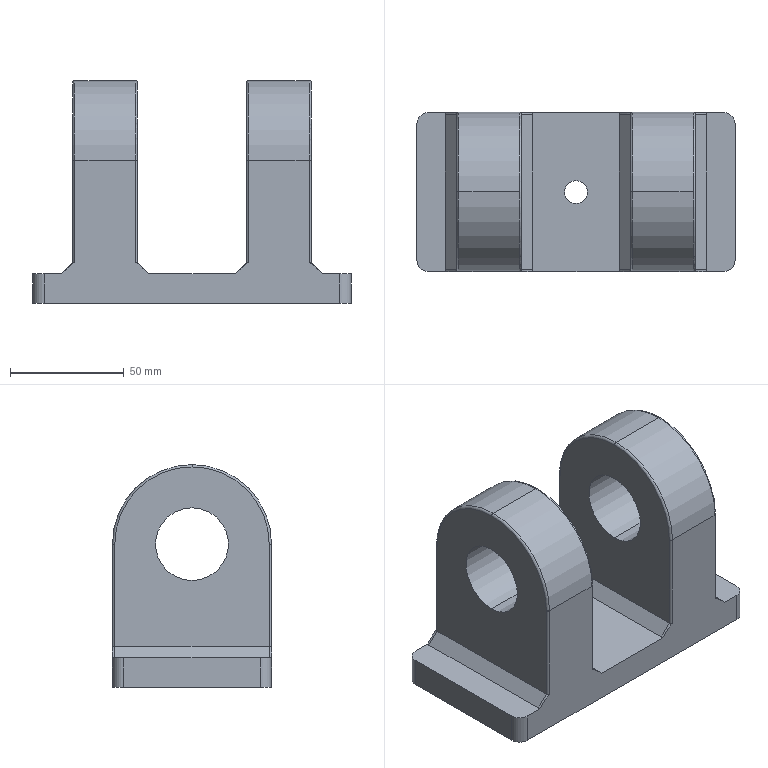Part | STEP file | Frame R-pair hinge lug | 1 solid | 52 faces | box 140 x 70 x 98 mm | volume 392765 mm3 | cylinder 22 | plane 16 | cone 8 | torus 6 | commonest cylinder face diameters 2 x8 10 x6 32 x4 70 x4